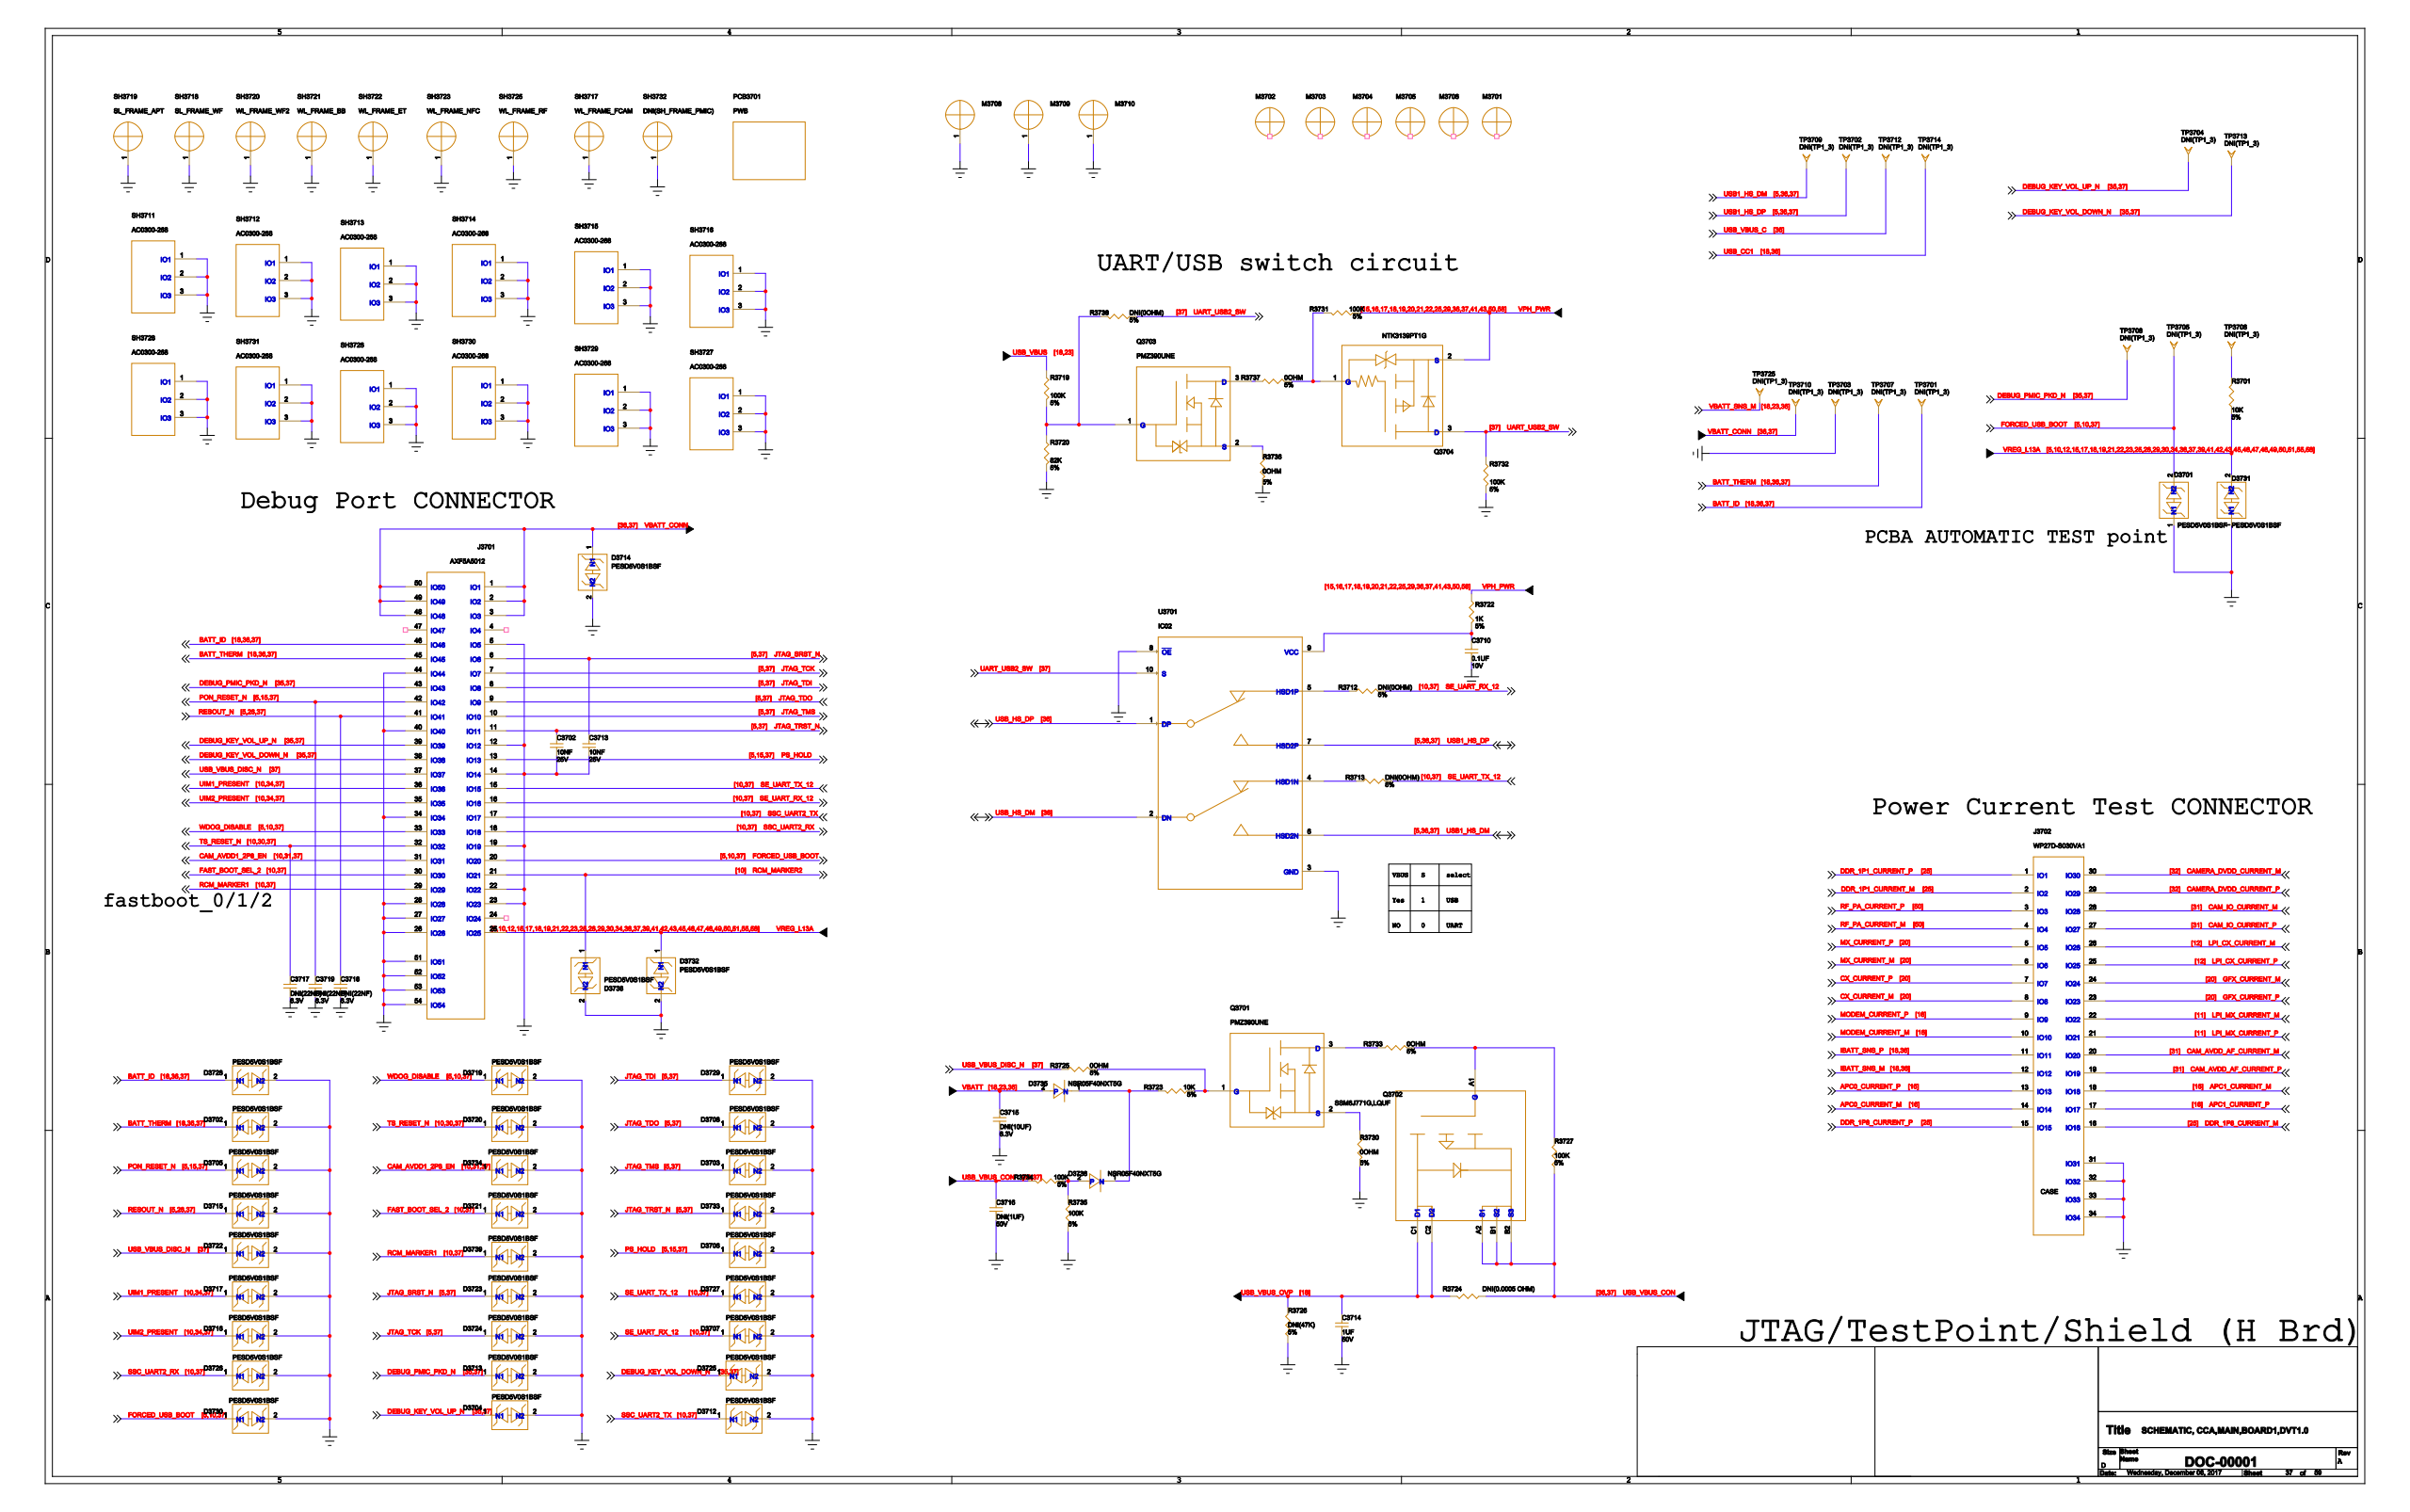Circuit board | KiCad | 1657 parts | 1365 nets | one sheet of the schematic
Parts on this sheet (reference | value | footprint):
C3702
C3710
C3713
C3714
C3715
C3716
C3717
C3718
C3719
D3701
D3702
D3703
D3704
D3705
D3706
D3707
D3708
D3712
D3713
D3714
D3715
D3716
D3717
D3719
D3720
D3721
D3722
D3723
D3724
D3725
D3726
D3727
D3728
D3729
D3730
D3731
D3732
D3733
D3734
D3735
D3736
D3738
D3739
J3701
J3702
M3701
M3702
M3703
M3704
M3705
M3706
M3708
M3709
M3710
Q3701
Q3702
Q3703
Q3704
R3701
R3712
R3713
R3719
R3720
R3722
R3723
R3724
R3725
R3726
R3727
R3730
R3731
R3732
R3733
R3734
R3735
R3736
R3737
R3738
SH3711
SH3712
SH3713
SH3714
SH3715
SH3716
SH3717
SH3718
SH3719
SH3720
SH3721
SH3722
SH3723
SH3725
SH3726
SH3727
SH3728
SH3729
SH3730
SH3731
SH3732
TP3701
TP3702
TP3703
TP3704
TP3705
TP3706
TP3707
TP3708
TP3709
TP3710
TP3712
TP3713
TP3714
TP3725
U3701
Nets of these parts (net: part-pin ...):
GND: C3702-1 C3710-2 C3713-1 C3714-2 C3715-2 C3716-2 C3717-2 C3718-2 C3719-2 D3701-1 D3702-2 D3703-2 D3704-2 D3705-2 D3706-2 D3707-2 D3708-2 D3712-2 D3713-2 D3714-2 D3715-2 D3716-2 D3717-2 D3719-2 D3720-2 D3721-2 D3722-2 D3723-2 D3724-2 D3725-2 D3726-2 D3727-2 D3728-2 D3729-2 D3730-2 D3731-1 D3732-2 D3733-2 D3734-2 D3738-2 D3739-2 M3708-1 M3709-1 M3710-1 R3720-1 R3726-2 R3730-1 R3732-1 R3735-1 R3736-1 SH3711-1 SH3711-2 SH3711-3 SH3712-1 SH3712-2 SH3712-3 SH3713-1 SH3713-2 SH3713-3 SH3714-1 SH3714-2 SH3714-3 SH3715-1 SH3715-2 SH3715-3 SH3716-1 SH3716-2 SH3716-3 SH3717-1 SH3718-1 SH3719-1 SH3720-1 SH3721-1 SH3722-1 SH3723-1 SH3725-1 SH3726-1 SH3726-2 SH3726-3 SH3727-1 SH3727-2 SH3727-3 SH3728-1 SH3728-2 SH3728-3 SH3729-1 SH3729-2 SH3729-3 SH3730-1 SH3730-2 SH3730-3 SH3731-1 SH3731-2 SH3731-3 SH3732-1 TP3703-1 U3701-3 U3701-8 J3701-5 J3701-12 J3701-14 J3701-19 J3701-22 J3701-23 J3701-26 J3701-27 J3701-28 J3701-34 J3701-40 J3701-44 J3701-51 J3701-52 J3701-53 J3701-54 J3702-31 J3702-32 J3702-33 J3702-34
RESOUT_N: C3718-1 D3715-1 J3701-41
VREG_L13A: D3731-2 D3732-1 R3701-2 J3701-25
VPH_PWR: Q3704-2 R3722-2 R3731-2
BATT_THERM: D3702-1 TP3707-1 J3701-45
APC0_CURRENT_P: J3702-13
N25038074: D3735-1 D3736-1 R3723-1
N25038026: Q3701-1 R3723-2 R3725-1
USB_VBUS_CON: C3716-1 Q3702-A2 Q3702-B1 Q3702-B2 R3724-2 R3727-2 R3734-1
N25038107: D3736-2 R3734-2 R3735-2
N25036419: Q3703-1 R3719-1 R3720-2 R3738-1
UART_USB2_SW: Q3704-3 R3732-2 R3738-2 U3701-10
N25038024: Q3702-A1 R3727-1 R3733-1
USB_VBUS_OVP: C3714-1 Q3702-C1 Q3702-C2 R3724-1 R3726-1
USB1_HS_DP: TP3702-1 U3701-7
USB_HS_DP: U3701-1
USB_HS_DM: U3701-2
N25036614: R3713-2 U3701-4
N25036600: R3712-2 U3701-5
USB1_HS_DM: TP3709-1 U3701-6
N25036707: C3710-1 R3722-1 U3701-9
USB_VBUS: R3719-2
N25036456: Q3703-2 R3736-2
N25036428: Q3704-1 R3731-1 R3737-1
TS_RESET_N: C3717-1 D3720-1 J3701-32
VBATT_CONN: D3714-1 TP3710-1 J3701-1 J3701-2 J3701-3 J3701-48 J3701-49 J3701-50
VBATT: C3715-1 D3735-2
WDOG_DISABLE: D3719-1 J3701-33
PON_RESET_N: C3719-1 D3705-1 J3701-42
IBATT_SNS_M: J3702-12
APC0_CURRENT_M: J3702-14
APC1_CURRENT_M: J3702-18
CX_CURRENT_M: J3702-8
USB_CC1: TP3714-1
M_AVDD1_2P8_EN: D3734-1 J3701-31
BATT_ID: D3728-1 TP3701-1 J3701-46
CX_CURRENT_P: J3702-7
PS_HOLD: D3706-1 J3701-13
NET_1263: M3705-1
UIM1_PRESENT: D3717-1 J3701-36
AST_BOOT_SEL_2: D3721-1 J3701-30
VBATT_SNS_M: TP3725-1
NET_1262: M3706-1
N25036430: Q3703-3 R3737-2
APC1_CURRENT_P: J3702-17
N25038263: Q3701-3 R3733-2
GFX_CURRENT_M: J3702-24
SSC_UART2_RX: D3726-1 J3701-18
SSC_UART2_TX: D3712-1 J3701-17
ORCED_USB_BOOT: D3701-2 D3730-1 TP3705-1 J3701-20
RCM_MARKER1: D3739-1 J3701-29
UIM2_PRESENT: D3716-1 J3701-35
SE_UART_RX_12: D3707-1 R3712-1 J3701-16
SE_UART_TX_12: D3727-1 R3713-1 J3701-15
JTAG_TDI: D3729-1 J3701-8
JTAG_TDO: D3708-1 J3701-9
JTAG_TCK: D3724-1 J3701-7
JTAG_TRST_N: C3702-2 D3733-1 J3701-11
JTAG_TMS: D3703-1 J3701-10
JTAG_SRST_N: C3713-2 D3723-1 J3701-6
RCM_MARKER2: D3738-1 J3701-21
N25038020: Q3701-2 R3730-2
MX_CURRENT_M: J3702-6
IBATT_SNS_P: J3702-11
USB_VBUS_C: TP3712-1
MX_CURRENT_P: J3702-5
GFX_CURRENT_P: J3702-23
NET_1264: M3704-1
SB_VBUS_DISC_N: D3722-1 R3725-2 J3701-37
BUG_PMIC_PKD_N: D3713-1 TP3708-1 J3701-43
NET_1266: M3702-1
G_KEY_VOL_UP_N: D3704-1 TP3704-1 J3701-39
N46423714: R3701-1 TP3706-1
KEY_VOL_DOWN_N: D3725-1 TP3713-1 J3701-38
NET_1267: M3701-1
NET_1265: M3703-1